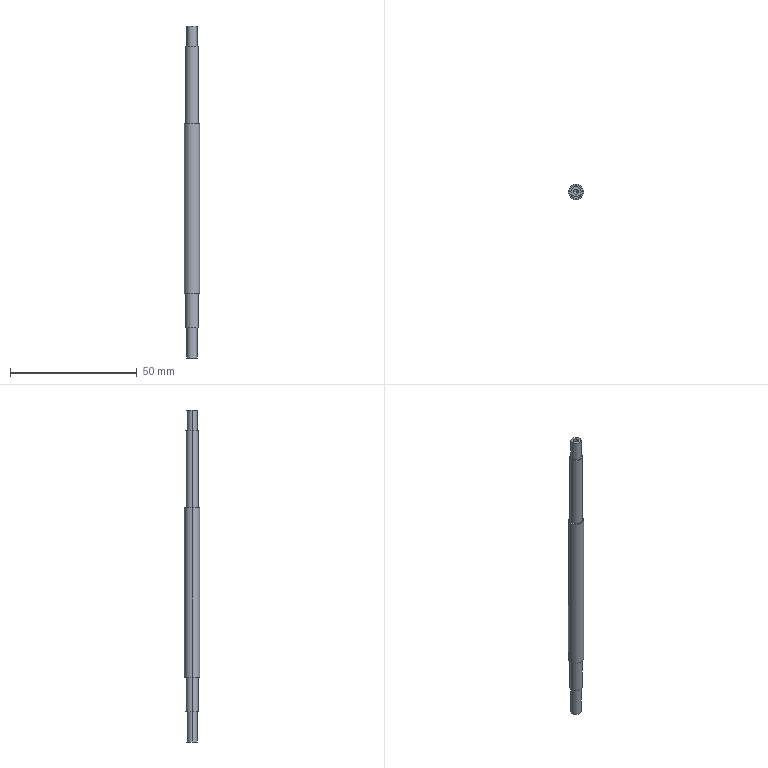Part | SolidWorks | features ICE 4, 3DProfileFeature 1, Extrusion 1, HoleWzd 1 | 1 solid | 20 faces | box 6 x 6 x 131 mm | volume 2988 mm3 | cylinder 12 | plane 6 | cone 2 | commonest cylinder face diameters 4 x4 5 x4 2.05 x2 6 x2
STEP:
#1=CARTESIAN_POINT('',(-1.025,0.,112.65));
#2=VERTEX_POINT('',#1);
#3=CARTESIAN_POINT('',(1.025,0.,112.65));
#4=VERTEX_POINT('',#3);
#5=CARTESIAN_POINT('',(0.,0.,112.65));
#6=DIRECTION('',(0.,0.,1.));
#7=DIRECTION('',(1.,0.,0.));
#8=AXIS2_PLACEMENT_3D('',#5,#6,#7);
#9=CIRCLE('',#8,1.025);
#10=EDGE_CURVE('',#2,#4,#9,.T.);
#11=ORIENTED_EDGE('',*,*,#10,.F.);
#12=CARTESIAN_POINT('',(-1.025,0.,119.));
#13=VERTEX_POINT('',#12);
#14=CARTESIAN_POINT('',(-1.025,0.,119.));
#15=DIRECTION('',(0.,0.,1.));
#16=VECTOR('',#15,1000.);
#17=LINE('',#14,#16);
#18=EDGE_CURVE('',#2,#13,#17,.T.);
#19=ORIENTED_EDGE('',*,*,#18,.T.);
#20=CARTESIAN_POINT('',(1.025,0.,119.));
#21=VERTEX_POINT('',#20);
#22=CARTESIAN_POINT('',(0.,0.,119.));
#23=DIRECTION('',(0.,0.,1.));
#24=DIRECTION('',(1.,0.,0.));
#25=AXIS2_PLACEMENT_3D('',#22,#23,#24);
#26=CIRCLE('',#25,1.025);
#27=EDGE_CURVE('',#13,#21,#26,.T.);
#28=ORIENTED_EDGE('',*,*,#27,.T.);
#29=CARTESIAN_POINT('',(1.025,0.,119.));
#30=DIRECTION('',(0.,0.,1.));
#31=VECTOR('',#30,1000.);
#32=LINE('',#29,#31);
#33=EDGE_CURVE('',#4,#21,#32,.T.);
#34=ORIENTED_EDGE('',*,*,#33,.F.);
#35=EDGE_LOOP('',(#11,#19,#28,#34));
#36=FACE_OUTER_BOUND('',#35,.T.);
#37=CARTESIAN_POINT('',(0.,0.,119.));
#38=DIRECTION('',(0.,0.,1.));
#39=DIRECTION('',(1.,0.,0.));
#40=AXIS2_PLACEMENT_3D('',#37,#38,#39);
#41=CYLINDRICAL_SURFACE('',#40,1.025);
#42=ADVANCED_FACE('',(#36),#41,.F.);
#43=CARTESIAN_POINT('',(0.,0.,112.034));
#44=VERTEX_POINT('',#43);
#45=CARTESIAN_POINT('',(1.025,0.,112.65));
#46=DIRECTION('',(0.8572,0.,0.515));
#47=VECTOR('',#46,1000.);
#48=LINE('',#45,#47);
#49=EDGE_CURVE('',#44,#4,#48,.T.);
#50=ORIENTED_EDGE('',*,*,#49,.F.);
#51=CARTESIAN_POINT('',(-1.025,0.,112.65));
#52=DIRECTION('',(-0.8572,0.,0.515));
#53=VECTOR('',#52,1000.);
#54=LINE('',#51,#53);
#55=EDGE_CURVE('',#44,#2,#54,.T.);
#56=ORIENTED_EDGE('',*,*,#55,.T.);
#57=ORIENTED_EDGE('',*,*,#10,.T.);
#58=EDGE_LOOP('',(#50,#56,#57));
#59=FACE_OUTER_BOUND('',#58,.T.);
#60=CARTESIAN_POINT('',(0.,0.,112.65));
#61=DIRECTION('',(0.,0.,1.));
#62=DIRECTION('',(1.,0.,0.));
#63=AXIS2_PLACEMENT_3D('',#60,#61,#62);
#64=CONICAL_SURFACE('',#63,1.025,1.03);
#65=ADVANCED_FACE('',(#59),#64,.F.);
#66=CARTESIAN_POINT('',(-2.,0.,-12.));
#67=VERTEX_POINT('',#66);
#68=CARTESIAN_POINT('',(2.,0.,-12.));
#69=VERTEX_POINT('',#68);
#70=CARTESIAN_POINT('',(0.,0.,-12.));
#71=DIRECTION('',(0.,0.,-1.));
#72=DIRECTION('',(-1.,0.,0.));
#73=AXIS2_PLACEMENT_3D('',#70,#71,#72);
#74=CIRCLE('',#73,2.);
#75=EDGE_CURVE('',#67,#69,#74,.T.);
#76=ORIENTED_EDGE('',*,*,#75,.F.);
#77=CARTESIAN_POINT('',(-2.,0.,0.));
#78=VERTEX_POINT('',#77);
#79=CARTESIAN_POINT('',(-2.,0.,-12.));
#80=DIRECTION('',(0.,0.,1.));
#81=VECTOR('',#80,1000.);
#82=LINE('',#79,#81);
#83=EDGE_CURVE('',#67,#78,#82,.T.);
#84=ORIENTED_EDGE('',*,*,#83,.T.);
#85=CARTESIAN_POINT('',(2.,0.,0.));
#86=VERTEX_POINT('',#85);
#87=CARTESIAN_POINT('',(0.,0.,0.));
#88=DIRECTION('',(0.,0.,-1.));
#89=DIRECTION('',(-1.,0.,0.));
#90=AXIS2_PLACEMENT_3D('',#87,#88,#89);
#91=CIRCLE('',#90,2.);
#92=EDGE_CURVE('',#78,#86,#91,.T.);
#93=ORIENTED_EDGE('',*,*,#92,.T.);
#94=CARTESIAN_POINT('',(2.,0.,-12.));
#95=DIRECTION('',(0.,0.,1.));
#96=VECTOR('',#95,1000.);
#97=LINE('',#94,#96);
#98=EDGE_CURVE('',#69,#86,#97,.T.);
#99=ORIENTED_EDGE('',*,*,#98,.F.);
#100=EDGE_LOOP('',(#76,#84,#93,#99));
#101=FACE_OUTER_BOUND('',#100,.T.);
#102=CARTESIAN_POINT('',(0.,0.,-12.));
#103=DIRECTION('',(0.,0.,1.));
#104=DIRECTION('',(1.,0.,0.));
#105=AXIS2_PLACEMENT_3D('',#102,#103,#104);
#106=CYLINDRICAL_SURFACE('',#105,2.);
#107=ADVANCED_FACE('',(#101),#106,.T.);
#108=CARTESIAN_POINT('',(2.,0.,119.));
#109=VERTEX_POINT('',#108);
#110=CARTESIAN_POINT('',(-2.,0.,119.));
#111=VERTEX_POINT('',#110);
#112=CARTESIAN_POINT('',(0.,0.,119.));
#113=DIRECTION('',(0.,0.,1.));
#114=DIRECTION('',(1.,0.,0.));
#115=AXIS2_PLACEMENT_3D('',#112,#113,#114);
#116=CIRCLE('',#115,2.);
#117=EDGE_CURVE('',#109,#111,#116,.T.);
#118=ORIENTED_EDGE('',*,*,#117,.F.);
#119=CARTESIAN_POINT('',(2.,0.,111.));
#120=VERTEX_POINT('',#119);
#121=CARTESIAN_POINT('',(2.,0.,119.));
#122=DIRECTION('',(0.,0.,-1.));
#123=VECTOR('',#122,1000.);
#124=LINE('',#121,#123);
#125=EDGE_CURVE('',#109,#120,#124,.T.);
#126=ORIENTED_EDGE('',*,*,#125,.T.);
#127=CARTESIAN_POINT('',(-2.,0.,111.));
#128=VERTEX_POINT('',#127);
#129=CARTESIAN_POINT('',(0.,0.,111.));
#130=DIRECTION('',(0.,0.,1.));
#131=DIRECTION('',(1.,0.,0.));
#132=AXIS2_PLACEMENT_3D('',#129,#130,#131);
#133=CIRCLE('',#132,2.);
#134=EDGE_CURVE('',#120,#128,#133,.T.);
#135=ORIENTED_EDGE('',*,*,#134,.T.);
#136=CARTESIAN_POINT('',(-2.,0.,119.));
#137=DIRECTION('',(0.,0.,-1.));
#138=VECTOR('',#137,1000.);
#139=LINE('',#136,#138);
#140=EDGE_CURVE('',#111,#128,#139,.T.);
#141=ORIENTED_EDGE('',*,*,#140,.F.);
#142=EDGE_LOOP('',(#118,#126,#135,#141));
#143=FACE_OUTER_BOUND('',#142,.T.);
#144=CARTESIAN_POINT('',(0.,0.,119.));
#145=DIRECTION('',(0.,0.,-1.));
#146=DIRECTION('',(-1.,0.,0.));
#147=AXIS2_PLACEMENT_3D('',#144,#145,#146);
#148=CYLINDRICAL_SURFACE('',#147,2.);
#149=ADVANCED_FACE('',(#143),#148,.T.);
#150=CARTESIAN_POINT('',(2.5,0.,111.));
#151=VERTEX_POINT('',#150);
#152=CARTESIAN_POINT('',(-2.5,0.,111.));
#153=VERTEX_POINT('',#152);
#154=CARTESIAN_POINT('',(0.,0.,111.));
#155=DIRECTION('',(0.,0.,1.));
#156=DIRECTION('',(1.,0.,0.));
#157=AXIS2_PLACEMENT_3D('',#154,#155,#156);
#158=CIRCLE('',#157,2.5);
#159=EDGE_CURVE('',#151,#153,#158,.T.);
#160=ORIENTED_EDGE('',*,*,#159,.F.);
#161=CARTESIAN_POINT('',(2.5,0.,80.5));
#162=VERTEX_POINT('',#161);
#163=CARTESIAN_POINT('',(2.5,0.,111.));
#164=DIRECTION('',(0.,0.,-1.));
#165=VECTOR('',#164,1000.);
#166=LINE('',#163,#165);
#167=EDGE_CURVE('',#151,#162,#166,.T.);
#168=ORIENTED_EDGE('',*,*,#167,.T.);
#169=CARTESIAN_POINT('',(-2.5,0.,80.5));
#170=VERTEX_POINT('',#169);
#171=CARTESIAN_POINT('',(0.,0.,80.5));
#172=DIRECTION('',(0.,0.,1.));
#173=DIRECTION('',(1.,0.,0.));
#174=AXIS2_PLACEMENT_3D('',#171,#172,#173);
#175=CIRCLE('',#174,2.5);
#176=EDGE_CURVE('',#162,#170,#175,.T.);
#177=ORIENTED_EDGE('',*,*,#176,.T.);
#178=CARTESIAN_POINT('',(-2.5,0.,111.));
#179=DIRECTION('',(0.,0.,-1.));
#180=VECTOR('',#179,1000.);
#181=LINE('',#178,#180);
#182=EDGE_CURVE('',#153,#170,#181,.T.);
#183=ORIENTED_EDGE('',*,*,#182,.F.);
#184=EDGE_LOOP('',(#160,#168,#177,#183));
#185=FACE_OUTER_BOUND('',#184,.T.);
#186=CARTESIAN_POINT('',(0.,0.,111.));
#187=DIRECTION('',(0.,0.,-1.));
#188=DIRECTION('',(-1.,0.,0.));
#189=AXIS2_PLACEMENT_3D('',#186,#187,#188);
#190=CYLINDRICAL_SURFACE('',#189,2.5);
#191=ADVANCED_FACE('',(#185),#190,.T.);
#192=CARTESIAN_POINT('',(3.,0.,80.5));
#193=VERTEX_POINT('',#192);
#194=CARTESIAN_POINT('',(-3.,0.,80.5));
#195=VERTEX_POINT('',#194);
#196=CARTESIAN_POINT('',(0.,0.,80.5));
#197=DIRECTION('',(0.,0.,1.));
#198=DIRECTION('',(1.,0.,0.));
#199=AXIS2_PLACEMENT_3D('',#196,#197,#198);
#200=CIRCLE('',#199,3.);
#201=EDGE_CURVE('',#193,#195,#200,.T.);
#202=ORIENTED_EDGE('',*,*,#201,.F.);
#203=CARTESIAN_POINT('',(3.,0.,13.5));
#204=VERTEX_POINT('',#203);
#205=CARTESIAN_POINT('',(3.,0.,80.5));
#206=DIRECTION('',(0.,0.,-1.));
#207=VECTOR('',#206,1000.);
#208=LINE('',#205,#207);
#209=EDGE_CURVE('',#193,#204,#208,.T.);
#210=ORIENTED_EDGE('',*,*,#209,.T.);
#211=CARTESIAN_POINT('',(-3.,0.,13.5));
#212=VERTEX_POINT('',#211);
#213=CARTESIAN_POINT('',(0.,0.,13.5));
#214=DIRECTION('',(0.,0.,1.));
#215=DIRECTION('',(1.,0.,0.));
#216=AXIS2_PLACEMENT_3D('',#213,#214,#215);
#217=CIRCLE('',#216,3.);
#218=EDGE_CURVE('',#204,#212,#217,.T.);
#219=ORIENTED_EDGE('',*,*,#218,.T.);
#220=CARTESIAN_POINT('',(-3.,0.,80.5));
#221=DIRECTION('',(0.,0.,-1.));
#222=VECTOR('',#221,1000.);
#223=LINE('',#220,#222);
#224=EDGE_CURVE('',#195,#212,#223,.T.);
#225=ORIENTED_EDGE('',*,*,#224,.F.);
#226=EDGE_LOOP('',(#202,#210,#219,#225));
#227=FACE_OUTER_BOUND('',#226,.T.);
#228=CARTESIAN_POINT('',(0.,0.,80.5));
#229=DIRECTION('',(0.,0.,-1.));
#230=DIRECTION('',(-1.,0.,0.));
#231=AXIS2_PLACEMENT_3D('',#228,#229,#230);
#232=CYLINDRICAL_SURFACE('',#231,3.);
#233=ADVANCED_FACE('',(#227),#232,.T.);
#234=CARTESIAN_POINT('',(2.5,0.,13.5));
#235=VERTEX_POINT('',#234);
#236=CARTESIAN_POINT('',(-2.5,0.,13.5));
#237=VERTEX_POINT('',#236);
#238=CARTESIAN_POINT('',(0.,0.,13.5));
#239=DIRECTION('',(0.,0.,1.));
#240=DIRECTION('',(1.,0.,0.));
#241=AXIS2_PLACEMENT_3D('',#238,#239,#240);
#242=CIRCLE('',#241,2.5);
#243=EDGE_CURVE('',#235,#237,#242,.T.);
#244=ORIENTED_EDGE('',*,*,#243,.F.);
#245=CARTESIAN_POINT('',(2.5,0.,0.));
#246=VERTEX_POINT('',#245);
#247=CARTESIAN_POINT('',(2.5,0.,13.5));
#248=DIRECTION('',(0.,0.,-1.));
#249=VECTOR('',#248,1000.);
#250=LINE('',#247,#249);
#251=EDGE_CURVE('',#235,#246,#250,.T.);
#252=ORIENTED_EDGE('',*,*,#251,.T.);
#253=CARTESIAN_POINT('',(-2.5,0.,0.));
#254=VERTEX_POINT('',#253);
#255=CARTESIAN_POINT('',(0.,0.,0.));
#256=DIRECTION('',(0.,0.,1.));
#257=DIRECTION('',(1.,0.,0.));
#258=AXIS2_PLACEMENT_3D('',#255,#256,#257);
#259=CIRCLE('',#258,2.5);
#260=EDGE_CURVE('',#246,#254,#259,.T.);
#261=ORIENTED_EDGE('',*,*,#260,.T.);
#262=CARTESIAN_POINT('',(-2.5,0.,13.5));
#263=DIRECTION('',(0.,0.,-1.));
#264=VECTOR('',#263,1000.);
#265=LINE('',#262,#264);
#266=EDGE_CURVE('',#237,#254,#265,.T.);
#267=ORIENTED_EDGE('',*,*,#266,.F.);
#268=EDGE_LOOP('',(#244,#252,#261,#267));
#269=FACE_OUTER_BOUND('',#268,.T.);
#270=CARTESIAN_POINT('',(0.,0.,13.5));
#271=DIRECTION('',(0.,0.,-1.));
#272=DIRECTION('',(-1.,0.,0.));
#273=AXIS2_PLACEMENT_3D('',#270,#271,#272);
#274=CYLINDRICAL_SURFACE('',#273,2.5);
#275=ADVANCED_FACE('',(#269),#274,.T.);
#276=ORIENTED_EDGE('',*,*,#251,.F.);
#277=CARTESIAN_POINT('',(0.,0.,13.5));
#278=DIRECTION('',(0.,0.,1.));
#279=DIRECTION('',(1.,0.,0.));
#280=AXIS2_PLACEMENT_3D('',#277,#278,#279);
#281=CIRCLE('',#280,2.5);
#282=EDGE_CURVE('',#237,#235,#281,.T.);
#283=ORIENTED_EDGE('',*,*,#282,.F.);
#284=ORIENTED_EDGE('',*,*,#266,.T.);
#285=CARTESIAN_POINT('',(0.,0.,0.));
#286=DIRECTION('',(0.,0.,1.));
#287=DIRECTION('',(1.,0.,0.));
#288=AXIS2_PLACEMENT_3D('',#285,#286,#287);
#289=CIRCLE('',#288,2.5);
#290=EDGE_CURVE('',#254,#246,#289,.T.);
#291=ORIENTED_EDGE('',*,*,#290,.T.);
#292=EDGE_LOOP('',(#276,#283,#284,#291));
#293=FACE_OUTER_BOUND('',#292,.T.);
#294=CARTESIAN_POINT('',(0.,0.,13.5));
#295=DIRECTION('',(0.,0.,-1.));
#296=DIRECTION('',(-1.,0.,0.));
#297=AXIS2_PLACEMENT_3D('',#294,#295,#296);
#298=CYLINDRICAL_SURFACE('',#297,2.5);
#299=ADVANCED_FACE('',(#293),#298,.T.);
#300=CARTESIAN_POINT('',(0.,0.,0.));
#301=DIRECTION('',(0.,0.,-1.));
#302=DIRECTION('',(-1.,0.,0.));
#303=AXIS2_PLACEMENT_3D('',#300,#301,#302);
#304=CIRCLE('',#303,2.);
#305=EDGE_CURVE('',#86,#78,#304,.T.);
#306=ORIENTED_EDGE('',*,*,#305,.F.);
#307=ORIENTED_EDGE('',*,*,#92,.F.);
#308=EDGE_LOOP('',(#306,#307));
#309=FACE_BOUND('',#308,.T.);
#310=ORIENTED_EDGE('',*,*,#290,.F.);
#311=ORIENTED_EDGE('',*,*,#260,.F.);
#312=EDGE_LOOP('',(#310,#311));
#313=FACE_OUTER_BOUND('',#312,.T.);
#314=CARTESIAN_POINT('',(0.,0.,0.));
#315=DIRECTION('',(0.,0.,1.));
#316=DIRECTION('',(1.,0.,0.));
#317=AXIS2_PLACEMENT_3D('',#314,#315,#316);
#318=PLANE('',#317);
#319=ADVANCED_FACE('',(#309,#313),#318,.F.);
#320=ORIENTED_EDGE('',*,*,#209,.F.);
#321=CARTESIAN_POINT('',(0.,0.,80.5));
#322=DIRECTION('',(0.,0.,1.));
#323=DIRECTION('',(1.,0.,0.));
#324=AXIS2_PLACEMENT_3D('',#321,#322,#323);
#325=CIRCLE('',#324,3.);
#326=EDGE_CURVE('',#195,#193,#325,.T.);
#327=ORIENTED_EDGE('',*,*,#326,.F.);
#328=ORIENTED_EDGE('',*,*,#224,.T.);
#329=CARTESIAN_POINT('',(0.,0.,13.5));
#330=DIRECTION('',(0.,0.,1.));
#331=DIRECTION('',(1.,0.,0.));
#332=AXIS2_PLACEMENT_3D('',#329,#330,#331);
#333=CIRCLE('',#332,3.);
#334=EDGE_CURVE('',#212,#204,#333,.T.);
#335=ORIENTED_EDGE('',*,*,#334,.T.);
#336=EDGE_LOOP('',(#320,#327,#328,#335));
#337=FACE_OUTER_BOUND('',#336,.T.);
#338=CARTESIAN_POINT('',(0.,0.,80.5));
#339=DIRECTION('',(0.,0.,-1.));
#340=DIRECTION('',(-1.,0.,0.));
#341=AXIS2_PLACEMENT_3D('',#338,#339,#340);
#342=CYLINDRICAL_SURFACE('',#341,3.);
#343=ADVANCED_FACE('',(#337),#342,.T.);
#344=CARTESIAN_POINT('',(0.,0.,80.5));
#345=DIRECTION('',(0.,0.,1.));
#346=DIRECTION('',(1.,0.,0.));
#347=AXIS2_PLACEMENT_3D('',#344,#345,#346);
#348=CIRCLE('',#347,2.5);
#349=EDGE_CURVE('',#170,#162,#348,.T.);
#350=ORIENTED_EDGE('',*,*,#349,.F.);
#351=ORIENTED_EDGE('',*,*,#176,.F.);
#352=EDGE_LOOP('',(#350,#351));
#353=FACE_BOUND('',#352,.T.);
#354=ORIENTED_EDGE('',*,*,#326,.T.);
#355=ORIENTED_EDGE('',*,*,#201,.T.);
#356=EDGE_LOOP('',(#354,#355));
#357=FACE_OUTER_BOUND('',#356,.T.);
#358=CARTESIAN_POINT('',(0.,0.,80.5));
#359=DIRECTION('',(0.,0.,1.));
#360=DIRECTION('',(1.,0.,0.));
#361=AXIS2_PLACEMENT_3D('',#358,#359,#360);
#362=PLANE('',#361);
#363=ADVANCED_FACE('',(#353,#357),#362,.T.);
#364=ORIENTED_EDGE('',*,*,#282,.T.);
#365=ORIENTED_EDGE('',*,*,#243,.T.);
#366=EDGE_LOOP('',(#364,#365));
#367=FACE_BOUND('',#366,.T.);
#368=ORIENTED_EDGE('',*,*,#334,.F.);
#369=ORIENTED_EDGE('',*,*,#218,.F.);
#370=EDGE_LOOP('',(#368,#369));
#371=FACE_OUTER_BOUND('',#370,.T.);
#372=CARTESIAN_POINT('',(0.,0.,13.5));
#373=DIRECTION('',(0.,0.,1.));
#374=DIRECTION('',(1.,0.,0.));
#375=AXIS2_PLACEMENT_3D('',#372,#373,#374);
#376=PLANE('',#375);
#377=ADVANCED_FACE('',(#367,#371),#376,.F.);
#378=ORIENTED_EDGE('',*,*,#167,.F.);
#379=CARTESIAN_POINT('',(0.,0.,111.));
#380=DIRECTION('',(0.,0.,1.));
#381=DIRECTION('',(1.,0.,0.));
#382=AXIS2_PLACEMENT_3D('',#379,#380,#381);
#383=CIRCLE('',#382,2.5);
#384=EDGE_CURVE('',#153,#151,#383,.T.);
#385=ORIENTED_EDGE('',*,*,#384,.F.);
#386=ORIENTED_EDGE('',*,*,#182,.T.);
#387=ORIENTED_EDGE('',*,*,#349,.T.);
#388=EDGE_LOOP('',(#378,#385,#386,#387));
#389=FACE_OUTER_BOUND('',#388,.T.);
#390=CARTESIAN_POINT('',(0.,0.,111.));
#391=DIRECTION('',(0.,0.,-1.));
#392=DIRECTION('',(-1.,0.,0.));
#393=AXIS2_PLACEMENT_3D('',#390,#391,#392);
#394=CYLINDRICAL_SURFACE('',#393,2.5);
#395=ADVANCED_FACE('',(#389),#394,.T.);
#396=CARTESIAN_POINT('',(0.,0.,111.));
#397=DIRECTION('',(0.,0.,1.));
#398=DIRECTION('',(1.,0.,0.));
#399=AXIS2_PLACEMENT_3D('',#396,#397,#398);
#400=CIRCLE('',#399,2.);
#401=EDGE_CURVE('',#128,#120,#400,.T.);
#402=ORIENTED_EDGE('',*,*,#401,.F.);
#403=ORIENTED_EDGE('',*,*,#134,.F.);
#404=EDGE_LOOP('',(#402,#403));
#405=FACE_BOUND('',#404,.T.);
#406=ORIENTED_EDGE('',*,*,#384,.T.);
#407=ORIENTED_EDGE('',*,*,#159,.T.);
#408=EDGE_LOOP('',(#406,#407));
#409=FACE_OUTER_BOUND('',#408,.T.);
#410=CARTESIAN_POINT('',(0.,0.,111.));
#411=DIRECTION('',(0.,0.,1.));
#412=DIRECTION('',(1.,0.,0.));
#413=AXIS2_PLACEMENT_3D('',#410,#411,#412);
#414=PLANE('',#413);
#415=ADVANCED_FACE('',(#405,#409),#414,.T.);
#416=ORIENTED_EDGE('',*,*,#125,.F.);
#417=CARTESIAN_POINT('',(0.,0.,119.));
#418=DIRECTION('',(0.,0.,1.));
#419=DIRECTION('',(1.,0.,0.));
#420=AXIS2_PLACEMENT_3D('',#417,#418,#419);
#421=CIRCLE('',#420,2.);
#422=EDGE_CURVE('',#111,#109,#421,.T.);
#423=ORIENTED_EDGE('',*,*,#422,.F.);
#424=ORIENTED_EDGE('',*,*,#140,.T.);
#425=ORIENTED_EDGE('',*,*,#401,.T.);
#426=EDGE_LOOP('',(#416,#423,#424,#425));
#427=FACE_OUTER_BOUND('',#426,.T.);
#428=CARTESIAN_POINT('',(0.,0.,119.));
#429=DIRECTION('',(0.,0.,-1.));
#430=DIRECTION('',(-1.,0.,0.));
#431=AXIS2_PLACEMENT_3D('',#428,#429,#430);
#432=CYLINDRICAL_SURFACE('',#431,2.);
#433=ADVANCED_FACE('',(#427),#432,.T.);
#434=CARTESIAN_POINT('',(0.,0.,119.));
#435=DIRECTION('',(0.,0.,1.));
#436=DIRECTION('',(1.,0.,0.));
#437=AXIS2_PLACEMENT_3D('',#434,#435,#436);
#438=CIRCLE('',#437,1.025);
#439=EDGE_CURVE('',#21,#13,#438,.T.);
#440=ORIENTED_EDGE('',*,*,#439,.F.);
#441=ORIENTED_EDGE('',*,*,#27,.F.);
#442=EDGE_LOOP('',(#440,#441));
#443=FACE_BOUND('',#442,.T.);
#444=ORIENTED_EDGE('',*,*,#422,.T.);
#445=ORIENTED_EDGE('',*,*,#117,.T.);
#446=EDGE_LOOP('',(#444,#445));
#447=FACE_OUTER_BOUND('',#446,.T.);
#448=CARTESIAN_POINT('',(0.,0.,119.));
#449=DIRECTION('',(0.,0.,1.));
#450=DIRECTION('',(1.,0.,0.));
#451=AXIS2_PLACEMENT_3D('',#448,#449,#450);
#452=PLANE('',#451);
#453=ADVANCED_FACE('',(#443,#447),#452,.T.);
#454=ORIENTED_EDGE('',*,*,#83,.F.);
#455=CARTESIAN_POINT('',(0.,0.,-12.));
#456=DIRECTION('',(0.,0.,-1.));
#457=DIRECTION('',(-1.,0.,0.));
#458=AXIS2_PLACEMENT_3D('',#455,#456,#457);
#459=CIRCLE('',#458,2.);
#460=EDGE_CURVE('',#69,#67,#459,.T.);
#461=ORIENTED_EDGE('',*,*,#460,.F.);
#462=ORIENTED_EDGE('',*,*,#98,.T.);
#463=ORIENTED_EDGE('',*,*,#305,.T.);
#464=EDGE_LOOP('',(#454,#461,#462,#463));
#465=FACE_OUTER_BOUND('',#464,.T.);
#466=CARTESIAN_POINT('',(0.,0.,-12.));
#467=DIRECTION('',(0.,0.,1.));
#468=DIRECTION('',(1.,0.,0.));
#469=AXIS2_PLACEMENT_3D('',#466,#467,#468);
#470=CYLINDRICAL_SURFACE('',#469,2.);
#471=ADVANCED_FACE('',(#465),#470,.T.);
#472=ORIENTED_EDGE('',*,*,#460,.T.);
#473=ORIENTED_EDGE('',*,*,#75,.T.);
#474=EDGE_LOOP('',(#472,#473));
#475=FACE_OUTER_BOUND('',#474,.T.);
#476=CARTESIAN_POINT('',(0.,0.,-12.));
#477=DIRECTION('',(0.,0.,-1.));
#478=DIRECTION('',(-1.,0.,0.));
#479=AXIS2_PLACEMENT_3D('',#476,#477,#478);
#480=PLANE('',#479);
#481=ADVANCED_FACE('',(#475),#480,.T.);
#482=ORIENTED_EDGE('',*,*,#55,.F.);
#483=ORIENTED_EDGE('',*,*,#49,.T.);
#484=CARTESIAN_POINT('',(0.,0.,112.65));
#485=DIRECTION('',(0.,0.,1.));
#486=DIRECTION('',(1.,0.,0.));
#487=AXIS2_PLACEMENT_3D('',#484,#485,#486);
#488=CIRCLE('',#487,1.025);
#489=EDGE_CURVE('',#4,#2,#488,.T.);
#490=ORIENTED_EDGE('',*,*,#489,.T.);
#491=EDGE_LOOP('',(#482,#483,#490));
#492=FACE_OUTER_BOUND('',#491,.T.);
#493=CARTESIAN_POINT('',(0.,0.,112.65));
#494=DIRECTION('',(0.,0.,1.));
#495=DIRECTION('',(1.,0.,0.));
#496=AXIS2_PLACEMENT_3D('',#493,#494,#495);
#497=CONICAL_SURFACE('',#496,1.025,1.03);
#498=ADVANCED_FACE('',(#492),#497,.F.);
#499=ORIENTED_EDGE('',*,*,#18,.F.);
#500=ORIENTED_EDGE('',*,*,#489,.F.);
#501=ORIENTED_EDGE('',*,*,#33,.T.);
#502=ORIENTED_EDGE('',*,*,#439,.T.);
#503=EDGE_LOOP('',(#499,#500,#501,#502));
#504=FACE_OUTER_BOUND('',#503,.T.);
#505=CARTESIAN_POINT('',(0.,0.,119.));
#506=DIRECTION('',(0.,0.,1.));
#507=DIRECTION('',(1.,0.,0.));
#508=AXIS2_PLACEMENT_3D('',#505,#506,#507);
#509=CYLINDRICAL_SURFACE('',#508,1.025);
#510=ADVANCED_FACE('',(#504),#509,.F.);
#511=CLOSED_SHELL('',(#42,#65,#107,#149,#191,#233,#275,#299,#319,#343,#363,#377,#395,#415,#433,#453,#471,#481,#498,#510));
#512=MANIFOLD_SOLID_BREP('',#511);
#513=CARTESIAN_POINT('',(0.,0.,0.));
#514=DIRECTION('',(0.,0.,1.));
#515=DIRECTION('',(1.,0.,0.));
#516=AXIS2_PLACEMENT_3D('',#513,#514,#515);
#517=(LENGTH_UNIT()NAMED_UNIT(*)SI_UNIT(.MILLI.,.METRE.));
#518=UNCERTAINTY_MEASURE_WITH_UNIT(LENGTH_MEASURE(0.00001),#517,'','');
#519=(NAMED_UNIT(*)PLANE_ANGLE_UNIT()SI_UNIT($,.RADIAN.));
#520=(NAMED_UNIT(*)SI_UNIT($,.STERADIAN.)SOLID_ANGLE_UNIT());
#521=(GEOMETRIC_REPRESENTATION_CONTEXT(3)GLOBAL_UNCERTAINTY_ASSIGNED_CONTEXT((#518))GLOBAL_UNIT_ASSIGNED_CONTEXT((#517,#519,#520))REPRESENTATION_CONTEXT('',''));
#522=ADVANCED_BREP_SHAPE_REPRESENTATION('',(#512,#516),#521);